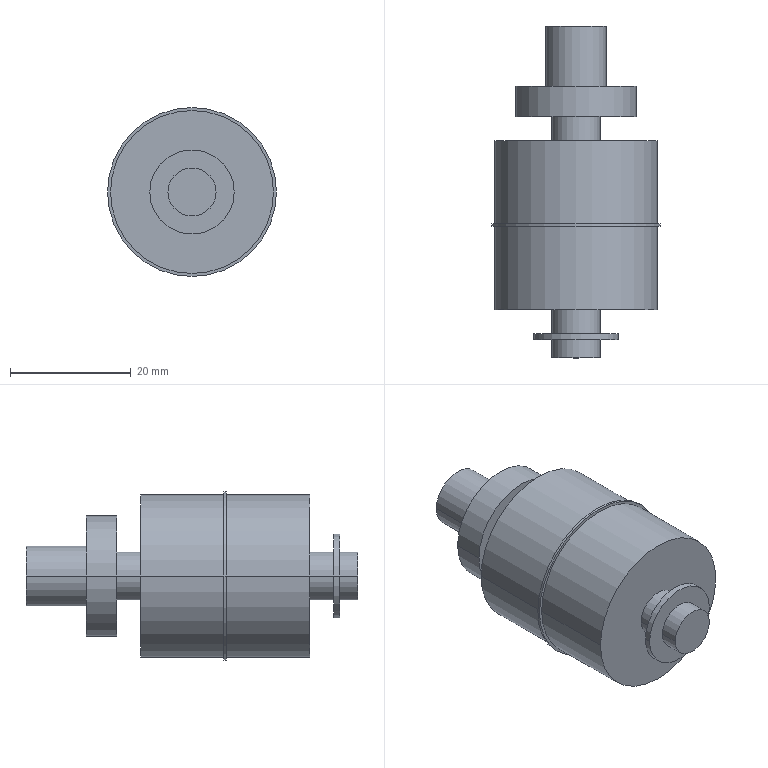Part | SolidWorks | features Revolution 1 | 1 solid | 28 faces | box 28 x 55 x 28 mm | volume 19112 mm3 | cylinder 18 | plane 10 | commonest cylinder face diameters 8 x6 27 x4 10 x2 14 x2 20 x2 28 x2
STEP:
#1=CARTESIAN_POINT('',(14.,22.2,0.));
#2=VERTEX_POINT('',#1);
#3=CARTESIAN_POINT('',(-14.,22.2,0.));
#4=VERTEX_POINT('',#3);
#5=CARTESIAN_POINT('',(0.,22.2,0.));
#6=DIRECTION('',(0.,-1.,0.));
#7=DIRECTION('',(1.,0.,0.));
#8=AXIS2_PLACEMENT_3D('',#5,#6,#7);
#9=CIRCLE('',#8,14.);
#10=EDGE_CURVE('',#2,#4,#9,.T.);
#11=ORIENTED_EDGE('',*,*,#10,.T.);
#12=CARTESIAN_POINT('',(-14.,21.8,0.));
#13=VERTEX_POINT('',#12);
#14=CARTESIAN_POINT('',(-14.,0.,0.));
#15=DIRECTION('',(0.,-1.,0.));
#16=VECTOR('',#15,1000.);
#17=LINE('',#14,#16);
#18=EDGE_CURVE('',#4,#13,#17,.T.);
#19=ORIENTED_EDGE('',*,*,#18,.T.);
#20=CARTESIAN_POINT('',(14.,21.8,0.));
#21=VERTEX_POINT('',#20);
#22=CARTESIAN_POINT('',(0.,21.8,0.));
#23=DIRECTION('',(0.,-1.,0.));
#24=DIRECTION('',(1.,0.,0.));
#25=AXIS2_PLACEMENT_3D('',#22,#23,#24);
#26=CIRCLE('',#25,14.);
#27=EDGE_CURVE('',#21,#13,#26,.T.);
#28=ORIENTED_EDGE('',*,*,#27,.F.);
#29=CARTESIAN_POINT('',(14.,0.,0.));
#30=DIRECTION('',(0.,-1.,0.));
#31=VECTOR('',#30,1000.);
#32=LINE('',#29,#31);
#33=EDGE_CURVE('',#2,#21,#32,.T.);
#34=ORIENTED_EDGE('',*,*,#33,.F.);
#35=EDGE_LOOP('',(#11,#19,#28,#34));
#36=FACE_OUTER_BOUND('',#35,.T.);
#37=CARTESIAN_POINT('',(0.,0.,0.));
#38=DIRECTION('',(0.,-1.,0.));
#39=DIRECTION('',(1.,0.,0.));
#40=AXIS2_PLACEMENT_3D('',#37,#38,#39);
#41=CYLINDRICAL_SURFACE('',#40,14.);
#42=ADVANCED_FACE('',(#36),#41,.T.);
#43=CARTESIAN_POINT('',(13.5,36.,0.));
#44=VERTEX_POINT('',#43);
#45=CARTESIAN_POINT('',(-13.5,36.,0.));
#46=VERTEX_POINT('',#45);
#47=CARTESIAN_POINT('',(0.,36.,0.));
#48=DIRECTION('',(0.,-1.,0.));
#49=DIRECTION('',(1.,0.,0.));
#50=AXIS2_PLACEMENT_3D('',#47,#48,#49);
#51=CIRCLE('',#50,13.5);
#52=EDGE_CURVE('',#44,#46,#51,.T.);
#53=ORIENTED_EDGE('',*,*,#52,.T.);
#54=CARTESIAN_POINT('',(-13.5,22.2,0.));
#55=VERTEX_POINT('',#54);
#56=CARTESIAN_POINT('',(-13.5,0.,0.));
#57=DIRECTION('',(0.,-1.,0.));
#58=VECTOR('',#57,1000.);
#59=LINE('',#56,#58);
#60=EDGE_CURVE('',#46,#55,#59,.T.);
#61=ORIENTED_EDGE('',*,*,#60,.T.);
#62=CARTESIAN_POINT('',(13.5,22.2,0.));
#63=VERTEX_POINT('',#62);
#64=CARTESIAN_POINT('',(0.,22.2,0.));
#65=DIRECTION('',(0.,-1.,0.));
#66=DIRECTION('',(1.,0.,0.));
#67=AXIS2_PLACEMENT_3D('',#64,#65,#66);
#68=CIRCLE('',#67,13.5);
#69=EDGE_CURVE('',#63,#55,#68,.T.);
#70=ORIENTED_EDGE('',*,*,#69,.F.);
#71=CARTESIAN_POINT('',(13.5,0.,0.));
#72=DIRECTION('',(0.,-1.,0.));
#73=VECTOR('',#72,1000.);
#74=LINE('',#71,#73);
#75=EDGE_CURVE('',#44,#63,#74,.T.);
#76=ORIENTED_EDGE('',*,*,#75,.F.);
#77=EDGE_LOOP('',(#53,#61,#70,#76));
#78=FACE_OUTER_BOUND('',#77,.T.);
#79=CARTESIAN_POINT('',(0.,0.,0.));
#80=DIRECTION('',(0.,-1.,0.));
#81=DIRECTION('',(1.,0.,0.));
#82=AXIS2_PLACEMENT_3D('',#79,#80,#81);
#83=CYLINDRICAL_SURFACE('',#82,13.5);
#84=ADVANCED_FACE('',(#78),#83,.T.);
#85=CARTESIAN_POINT('',(4.,40.,0.));
#86=VERTEX_POINT('',#85);
#87=CARTESIAN_POINT('',(-4.,40.,0.));
#88=VERTEX_POINT('',#87);
#89=CARTESIAN_POINT('',(0.,40.,0.));
#90=DIRECTION('',(0.,-1.,0.));
#91=DIRECTION('',(1.,0.,0.));
#92=AXIS2_PLACEMENT_3D('',#89,#90,#91);
#93=CIRCLE('',#92,4.);
#94=EDGE_CURVE('',#86,#88,#93,.T.);
#95=ORIENTED_EDGE('',*,*,#94,.T.);
#96=CARTESIAN_POINT('',(-4.,36.,0.));
#97=VERTEX_POINT('',#96);
#98=CARTESIAN_POINT('',(-4.,0.,0.));
#99=DIRECTION('',(0.,-1.,0.));
#100=VECTOR('',#99,1000.);
#101=LINE('',#98,#100);
#102=EDGE_CURVE('',#88,#97,#101,.T.);
#103=ORIENTED_EDGE('',*,*,#102,.T.);
#104=CARTESIAN_POINT('',(4.,36.,0.));
#105=VERTEX_POINT('',#104);
#106=CARTESIAN_POINT('',(0.,36.,0.));
#107=DIRECTION('',(0.,-1.,0.));
#108=DIRECTION('',(1.,0.,0.));
#109=AXIS2_PLACEMENT_3D('',#106,#107,#108);
#110=CIRCLE('',#109,4.);
#111=EDGE_CURVE('',#105,#97,#110,.T.);
#112=ORIENTED_EDGE('',*,*,#111,.F.);
#113=CARTESIAN_POINT('',(4.,0.,0.));
#114=DIRECTION('',(0.,-1.,0.));
#115=VECTOR('',#114,1000.);
#116=LINE('',#113,#115);
#117=EDGE_CURVE('',#86,#105,#116,.T.);
#118=ORIENTED_EDGE('',*,*,#117,.F.);
#119=EDGE_LOOP('',(#95,#103,#112,#118));
#120=FACE_OUTER_BOUND('',#119,.T.);
#121=CARTESIAN_POINT('',(0.,0.,0.));
#122=DIRECTION('',(0.,-1.,0.));
#123=DIRECTION('',(1.,0.,0.));
#124=AXIS2_PLACEMENT_3D('',#121,#122,#123);
#125=CYLINDRICAL_SURFACE('',#124,4.);
#126=ADVANCED_FACE('',(#120),#125,.T.);
#127=CARTESIAN_POINT('',(10.,45.,0.));
#128=VERTEX_POINT('',#127);
#129=CARTESIAN_POINT('',(-10.,45.,0.));
#130=VERTEX_POINT('',#129);
#131=CARTESIAN_POINT('',(0.,45.,0.));
#132=DIRECTION('',(0.,-1.,0.));
#133=DIRECTION('',(1.,0.,0.));
#134=AXIS2_PLACEMENT_3D('',#131,#132,#133);
#135=CIRCLE('',#134,10.);
#136=EDGE_CURVE('',#128,#130,#135,.T.);
#137=ORIENTED_EDGE('',*,*,#136,.T.);
#138=CARTESIAN_POINT('',(-10.,40.,0.));
#139=VERTEX_POINT('',#138);
#140=CARTESIAN_POINT('',(-10.,0.,0.));
#141=DIRECTION('',(0.,-1.,0.));
#142=VECTOR('',#141,1000.);
#143=LINE('',#140,#142);
#144=EDGE_CURVE('',#130,#139,#143,.T.);
#145=ORIENTED_EDGE('',*,*,#144,.T.);
#146=CARTESIAN_POINT('',(10.,40.,0.));
#147=VERTEX_POINT('',#146);
#148=CARTESIAN_POINT('',(0.,40.,0.));
#149=DIRECTION('',(0.,-1.,0.));
#150=DIRECTION('',(1.,0.,0.));
#151=AXIS2_PLACEMENT_3D('',#148,#149,#150);
#152=CIRCLE('',#151,10.);
#153=EDGE_CURVE('',#147,#139,#152,.T.);
#154=ORIENTED_EDGE('',*,*,#153,.F.);
#155=CARTESIAN_POINT('',(10.,0.,0.));
#156=DIRECTION('',(0.,-1.,0.));
#157=VECTOR('',#156,1000.);
#158=LINE('',#155,#157);
#159=EDGE_CURVE('',#128,#147,#158,.T.);
#160=ORIENTED_EDGE('',*,*,#159,.F.);
#161=EDGE_LOOP('',(#137,#145,#154,#160));
#162=FACE_OUTER_BOUND('',#161,.T.);
#163=CARTESIAN_POINT('',(0.,0.,0.));
#164=DIRECTION('',(0.,-1.,0.));
#165=DIRECTION('',(1.,0.,0.));
#166=AXIS2_PLACEMENT_3D('',#163,#164,#165);
#167=CYLINDRICAL_SURFACE('',#166,10.);
#168=ADVANCED_FACE('',(#162),#167,.T.);
#169=CARTESIAN_POINT('',(5.,55.,0.));
#170=VERTEX_POINT('',#169);
#171=CARTESIAN_POINT('',(-5.,55.,0.));
#172=VERTEX_POINT('',#171);
#173=CARTESIAN_POINT('',(0.,55.,0.));
#174=DIRECTION('',(0.,-1.,0.));
#175=DIRECTION('',(1.,0.,0.));
#176=AXIS2_PLACEMENT_3D('',#173,#174,#175);
#177=CIRCLE('',#176,5.);
#178=EDGE_CURVE('',#170,#172,#177,.T.);
#179=ORIENTED_EDGE('',*,*,#178,.T.);
#180=CARTESIAN_POINT('',(-5.,45.,0.));
#181=VERTEX_POINT('',#180);
#182=CARTESIAN_POINT('',(-5.,0.,0.));
#183=DIRECTION('',(0.,-1.,0.));
#184=VECTOR('',#183,1000.);
#185=LINE('',#182,#184);
#186=EDGE_CURVE('',#172,#181,#185,.T.);
#187=ORIENTED_EDGE('',*,*,#186,.T.);
#188=CARTESIAN_POINT('',(5.,45.,0.));
#189=VERTEX_POINT('',#188);
#190=CARTESIAN_POINT('',(0.,45.,0.));
#191=DIRECTION('',(0.,-1.,0.));
#192=DIRECTION('',(1.,0.,0.));
#193=AXIS2_PLACEMENT_3D('',#190,#191,#192);
#194=CIRCLE('',#193,5.);
#195=EDGE_CURVE('',#189,#181,#194,.T.);
#196=ORIENTED_EDGE('',*,*,#195,.F.);
#197=CARTESIAN_POINT('',(5.,0.,0.));
#198=DIRECTION('',(0.,-1.,0.));
#199=VECTOR('',#198,1000.);
#200=LINE('',#197,#199);
#201=EDGE_CURVE('',#170,#189,#200,.T.);
#202=ORIENTED_EDGE('',*,*,#201,.F.);
#203=EDGE_LOOP('',(#179,#187,#196,#202));
#204=FACE_OUTER_BOUND('',#203,.T.);
#205=CARTESIAN_POINT('',(0.,0.,0.));
#206=DIRECTION('',(0.,-1.,0.));
#207=DIRECTION('',(1.,0.,0.));
#208=AXIS2_PLACEMENT_3D('',#205,#206,#207);
#209=CYLINDRICAL_SURFACE('',#208,5.);
#210=ADVANCED_FACE('',(#204),#209,.T.);
#211=CARTESIAN_POINT('',(4.,3.,0.));
#212=VERTEX_POINT('',#211);
#213=CARTESIAN_POINT('',(-4.,3.,0.));
#214=VERTEX_POINT('',#213);
#215=CARTESIAN_POINT('',(0.,3.,0.));
#216=DIRECTION('',(0.,-1.,0.));
#217=DIRECTION('',(1.,0.,0.));
#218=AXIS2_PLACEMENT_3D('',#215,#216,#217);
#219=CIRCLE('',#218,4.);
#220=EDGE_CURVE('',#212,#214,#219,.T.);
#221=ORIENTED_EDGE('',*,*,#220,.T.);
#222=CARTESIAN_POINT('',(-4.,0.,0.));
#223=VERTEX_POINT('',#222);
#224=CARTESIAN_POINT('',(-4.,0.,0.));
#225=DIRECTION('',(0.,-1.,0.));
#226=VECTOR('',#225,1000.);
#227=LINE('',#224,#226);
#228=EDGE_CURVE('',#214,#223,#227,.T.);
#229=ORIENTED_EDGE('',*,*,#228,.T.);
#230=CARTESIAN_POINT('',(4.,0.,0.));
#231=VERTEX_POINT('',#230);
#232=CARTESIAN_POINT('',(0.,0.,0.));
#233=DIRECTION('',(0.,-1.,0.));
#234=DIRECTION('',(1.,0.,0.));
#235=AXIS2_PLACEMENT_3D('',#232,#233,#234);
#236=CIRCLE('',#235,4.);
#237=EDGE_CURVE('',#231,#223,#236,.T.);
#238=ORIENTED_EDGE('',*,*,#237,.F.);
#239=CARTESIAN_POINT('',(4.,0.,0.));
#240=DIRECTION('',(0.,-1.,0.));
#241=VECTOR('',#240,1000.);
#242=LINE('',#239,#241);
#243=EDGE_CURVE('',#212,#231,#242,.T.);
#244=ORIENTED_EDGE('',*,*,#243,.F.);
#245=EDGE_LOOP('',(#221,#229,#238,#244));
#246=FACE_OUTER_BOUND('',#245,.T.);
#247=CARTESIAN_POINT('',(0.,0.,0.));
#248=DIRECTION('',(0.,-1.,0.));
#249=DIRECTION('',(1.,0.,0.));
#250=AXIS2_PLACEMENT_3D('',#247,#248,#249);
#251=CYLINDRICAL_SURFACE('',#250,4.);
#252=ADVANCED_FACE('',(#246),#251,.T.);
#253=CARTESIAN_POINT('',(7.,4.,0.));
#254=VERTEX_POINT('',#253);
#255=CARTESIAN_POINT('',(-7.,4.,0.));
#256=VERTEX_POINT('',#255);
#257=CARTESIAN_POINT('',(0.,4.,0.));
#258=DIRECTION('',(0.,-1.,0.));
#259=DIRECTION('',(1.,0.,0.));
#260=AXIS2_PLACEMENT_3D('',#257,#258,#259);
#261=CIRCLE('',#260,7.);
#262=EDGE_CURVE('',#254,#256,#261,.T.);
#263=ORIENTED_EDGE('',*,*,#262,.T.);
#264=CARTESIAN_POINT('',(-7.,3.,0.));
#265=VERTEX_POINT('',#264);
#266=CARTESIAN_POINT('',(-7.,0.,0.));
#267=DIRECTION('',(0.,-1.,0.));
#268=VECTOR('',#267,1000.);
#269=LINE('',#266,#268);
#270=EDGE_CURVE('',#256,#265,#269,.T.);
#271=ORIENTED_EDGE('',*,*,#270,.T.);
#272=CARTESIAN_POINT('',(7.,3.,0.));
#273=VERTEX_POINT('',#272);
#274=CARTESIAN_POINT('',(0.,3.,0.));
#275=DIRECTION('',(0.,-1.,0.));
#276=DIRECTION('',(1.,0.,0.));
#277=AXIS2_PLACEMENT_3D('',#274,#275,#276);
#278=CIRCLE('',#277,7.);
#279=EDGE_CURVE('',#273,#265,#278,.T.);
#280=ORIENTED_EDGE('',*,*,#279,.F.);
#281=CARTESIAN_POINT('',(7.,0.,0.));
#282=DIRECTION('',(0.,-1.,0.));
#283=VECTOR('',#282,1000.);
#284=LINE('',#281,#283);
#285=EDGE_CURVE('',#254,#273,#284,.T.);
#286=ORIENTED_EDGE('',*,*,#285,.F.);
#287=EDGE_LOOP('',(#263,#271,#280,#286));
#288=FACE_OUTER_BOUND('',#287,.T.);
#289=CARTESIAN_POINT('',(0.,0.,0.));
#290=DIRECTION('',(0.,-1.,0.));
#291=DIRECTION('',(1.,0.,0.));
#292=AXIS2_PLACEMENT_3D('',#289,#290,#291);
#293=CYLINDRICAL_SURFACE('',#292,7.);
#294=ADVANCED_FACE('',(#288),#293,.T.);
#295=CARTESIAN_POINT('',(4.,8.,0.));
#296=VERTEX_POINT('',#295);
#297=CARTESIAN_POINT('',(-4.,8.,0.));
#298=VERTEX_POINT('',#297);
#299=CARTESIAN_POINT('',(0.,8.,0.));
#300=DIRECTION('',(0.,-1.,0.));
#301=DIRECTION('',(1.,0.,0.));
#302=AXIS2_PLACEMENT_3D('',#299,#300,#301);
#303=CIRCLE('',#302,4.);
#304=EDGE_CURVE('',#296,#298,#303,.T.);
#305=ORIENTED_EDGE('',*,*,#304,.T.);
#306=CARTESIAN_POINT('',(-4.,4.,0.));
#307=VERTEX_POINT('',#306);
#308=CARTESIAN_POINT('',(-4.,0.,0.));
#309=DIRECTION('',(0.,-1.,0.));
#310=VECTOR('',#309,1000.);
#311=LINE('',#308,#310);
#312=EDGE_CURVE('',#298,#307,#311,.T.);
#313=ORIENTED_EDGE('',*,*,#312,.T.);
#314=CARTESIAN_POINT('',(4.,4.,0.));
#315=VERTEX_POINT('',#314);
#316=CARTESIAN_POINT('',(0.,4.,0.));
#317=DIRECTION('',(0.,-1.,0.));
#318=DIRECTION('',(1.,0.,0.));
#319=AXIS2_PLACEMENT_3D('',#316,#317,#318);
#320=CIRCLE('',#319,4.);
#321=EDGE_CURVE('',#315,#307,#320,.T.);
#322=ORIENTED_EDGE('',*,*,#321,.F.);
#323=CARTESIAN_POINT('',(4.,0.,0.));
#324=DIRECTION('',(0.,-1.,0.));
#325=VECTOR('',#324,1000.);
#326=LINE('',#323,#325);
#327=EDGE_CURVE('',#296,#315,#326,.T.);
#328=ORIENTED_EDGE('',*,*,#327,.F.);
#329=EDGE_LOOP('',(#305,#313,#322,#328));
#330=FACE_OUTER_BOUND('',#329,.T.);
#331=CARTESIAN_POINT('',(0.,0.,0.));
#332=DIRECTION('',(0.,-1.,0.));
#333=DIRECTION('',(1.,0.,0.));
#334=AXIS2_PLACEMENT_3D('',#331,#332,#333);
#335=CYLINDRICAL_SURFACE('',#334,4.);
#336=ADVANCED_FACE('',(#330),#335,.T.);
#337=CARTESIAN_POINT('',(13.5,21.8,0.));
#338=VERTEX_POINT('',#337);
#339=CARTESIAN_POINT('',(-13.5,21.8,0.));
#340=VERTEX_POINT('',#339);
#341=CARTESIAN_POINT('',(0.,21.8,0.));
#342=DIRECTION('',(0.,-1.,0.));
#343=DIRECTION('',(1.,0.,0.));
#344=AXIS2_PLACEMENT_3D('',#341,#342,#343);
#345=CIRCLE('',#344,13.5);
#346=EDGE_CURVE('',#338,#340,#345,.T.);
#347=ORIENTED_EDGE('',*,*,#346,.T.);
#348=CARTESIAN_POINT('',(-13.5,8.,0.));
#349=VERTEX_POINT('',#348);
#350=CARTESIAN_POINT('',(-13.5,0.,0.));
#351=DIRECTION('',(0.,-1.,0.));
#352=VECTOR('',#351,1000.);
#353=LINE('',#350,#352);
#354=EDGE_CURVE('',#340,#349,#353,.T.);
#355=ORIENTED_EDGE('',*,*,#354,.T.);
#356=CARTESIAN_POINT('',(13.5,8.,0.));
#357=VERTEX_POINT('',#356);
#358=CARTESIAN_POINT('',(0.,8.,0.));
#359=DIRECTION('',(0.,-1.,0.));
#360=DIRECTION('',(1.,0.,0.));
#361=AXIS2_PLACEMENT_3D('',#358,#359,#360);
#362=CIRCLE('',#361,13.5);
#363=EDGE_CURVE('',#357,#349,#362,.T.);
#364=ORIENTED_EDGE('',*,*,#363,.F.);
#365=CARTESIAN_POINT('',(13.5,0.,0.));
#366=DIRECTION('',(0.,-1.,0.));
#367=VECTOR('',#366,1000.);
#368=LINE('',#365,#367);
#369=EDGE_CURVE('',#338,#357,#368,.T.);
#370=ORIENTED_EDGE('',*,*,#369,.F.);
#371=EDGE_LOOP('',(#347,#355,#364,#370));
#372=FACE_OUTER_BOUND('',#371,.T.);
#373=CARTESIAN_POINT('',(0.,0.,0.));
#374=DIRECTION('',(0.,-1.,0.));
#375=DIRECTION('',(1.,0.,0.));
#376=AXIS2_PLACEMENT_3D('',#373,#374,#375);
#377=CYLINDRICAL_SURFACE('',#376,13.5);
#378=ADVANCED_FACE('',(#372),#377,.T.);
#379=ORIENTED_EDGE('',*,*,#346,.F.);
#380=CARTESIAN_POINT('',(0.,21.8,0.));
#381=DIRECTION('',(0.,-1.,0.));
#382=DIRECTION('',(1.,0.,0.));
#383=AXIS2_PLACEMENT_3D('',#380,#381,#382);
#384=CIRCLE('',#383,13.5);
#385=EDGE_CURVE('',#340,#338,#384,.T.);
#386=ORIENTED_EDGE('',*,*,#385,.F.);
#387=EDGE_LOOP('',(#379,#386));
#388=FACE_BOUND('',#387,.T.);
#389=ORIENTED_EDGE('',*,*,#27,.T.);
#390=CARTESIAN_POINT('',(0.,21.8,0.));
#391=DIRECTION('',(0.,-1.,0.));
#392=DIRECTION('',(1.,0.,0.));
#393=AXIS2_PLACEMENT_3D('',#390,#391,#392);
#394=CIRCLE('',#393,14.);
#395=EDGE_CURVE('',#13,#21,#394,.T.);
#396=ORIENTED_EDGE('',*,*,#395,.T.);
#397=EDGE_LOOP('',(#389,#396));
#398=FACE_OUTER_BOUND('',#397,.T.);
#399=CARTESIAN_POINT('',(0.,21.8,0.));
#400=DIRECTION('',(0.,1.,0.));
#401=DIRECTION('',(-1.,0.,0.));
#402=AXIS2_PLACEMENT_3D('',#399,#400,#401);
#403=PLANE('',#402);
#404=ADVANCED_FACE('',(#388,#398),#403,.F.);
#405=ORIENTED_EDGE('',*,*,#354,.F.);
#406=ORIENTED_EDGE('',*,*,#385,.T.);
#407=ORIENTED_EDGE('',*,*,#369,.T.);
#408=CARTESIAN_POINT('',(0.,8.,0.));
#409=DIRECTION('',(0.,-1.,0.));
#410=DIRECTION('',(1.,0.,0.));
#411=AXIS2_PLACEMENT_3D('',#408,#409,#410);
#412=CIRCLE('',#411,13.5);
#413=EDGE_CURVE('',#349,#357,#412,.T.);
#414=ORIENTED_EDGE('',*,*,#413,.F.);
#415=EDGE_LOOP('',(#405,#406,#407,#414));
#416=FACE_OUTER_BOUND('',#415,.T.);
#417=CARTESIAN_POINT('',(0.,0.,0.));
#418=DIRECTION('',(0.,-1.,0.));
#419=DIRECTION('',(1.,0.,0.));
#420=AXIS2_PLACEMENT_3D('',#417,#418,#419);
#421=CYLINDRICAL_SURFACE('',#420,13.5);
#422=ADVANCED_FACE('',(#416),#421,.T.);
#423=ORIENTED_EDGE('',*,*,#304,.F.);
#424=CARTESIAN_POINT('',(0.,8.,0.));
#425=DIRECTION('',(0.,-1.,0.));
#426=DIRECTION('',(1.,0.,0.));
#427=AXIS2_PLACEMENT_3D('',#424,#425,#426);
#428=CIRCLE('',#427,4.);
#429=EDGE_CURVE('',#298,#296,#428,.T.);
#430=ORIENTED_EDGE('',*,*,#429,.F.);
#431=EDGE_LOOP('',(#423,#430));
#432=FACE_BOUND('',#431,.T.);
#433=ORIENTED_EDGE('',*,*,#363,.T.);
#434=ORIENTED_EDGE('',*,*,#413,.T.);
#435=EDGE_LOOP('',(#433,#434));
#436=FACE_OUTER_BOUND('',#435,.T.);
#437=CARTESIAN_POINT('',(0.,8.,0.));
#438=DIRECTION('',(0.,1.,0.));
#439=DIRECTION('',(-1.,0.,0.));
#440=AXIS2_PLACEMENT_3D('',#437,#438,#439);
#441=PLANE('',#440);
#442=ADVANCED_FACE('',(#432,#436),#441,.F.);
#443=ORIENTED_EDGE('',*,*,#312,.F.);
#444=ORIENTED_EDGE('',*,*,#429,.T.);
#445=ORIENTED_EDGE('',*,*,#327,.T.);
#446=CARTESIAN_POINT('',(0.,4.,0.));
#447=DIRECTION('',(0.,-1.,0.));
#448=DIRECTION('',(1.,0.,0.));
#449=AXIS2_PLACEMENT_3D('',#446,#447,#448);
#450=CIRCLE('',#449,4.);
#451=EDGE_CURVE('',#307,#315,#450,.T.);
#452=ORIENTED_EDGE('',*,*,#451,.F.);
#453=EDGE_LOOP('',(#443,#444,#445,#452));
#454=FACE_OUTER_BOUND('',#453,.T.);
#455=CARTESIAN_POINT('',(0.,0.,0.));
#456=DIRECTION('',(0.,-1.,0.));
#457=DIRECTION('',(1.,0.,0.));
#458=AXIS2_PLACEMENT_3D('',#455,#456,#457);
#459=CYLINDRICAL_SURFACE('',#458,4.);
#460=ADVANCED_FACE('',(#454),#459,.T.);
#461=ORIENTED_EDGE('',*,*,#262,.F.);
#462=CARTESIAN_POINT('',(0.,4.,0.));
#463=DIRECTION('',(0.,-1.,0.));
#464=DIRECTION('',(1.,0.,0.));
#465=AXIS2_PLACEMENT_3D('',#462,#463,#464);
#466=CIRCLE('',#465,7.);
#467=EDGE_CURVE('',#256,#254,#466,.T.);
#468=ORIENTED_EDGE('',*,*,#467,.F.);
#469=EDGE_LOOP('',(#461,#468));
#470=FACE_OUTER_BOUND('',#469,.T.);
#471=ORIENTED_EDGE('',*,*,#321,.T.);
#472=ORIENTED_EDGE('',*,*,#451,.T.);
#473=EDGE_LOOP('',(#471,#472));
#474=FACE_BOUND('',#473,.T.);
#475=CARTESIAN_POINT('',(0.,4.,0.));
#476=DIRECTION('',(0.,-1.,0.));
#477=DIRECTION('',(1.,0.,0.));
#478=AXIS2_PLACEMENT_3D('',#475,#476,#477);
#479=PLANE('',#478);
#480=ADVANCED_FACE('',(#470,#474),#479,.F.);
#481=ORIENTED_EDGE('',*,*,#270,.F.);
#482=ORIENTED_EDGE('',*,*,#467,.T.);
#483=ORIENTED_EDGE('',*,*,#285,.T.);
#484=CARTESIAN_POINT('',(0.,3.,0.));
#485=DIRECTION('',(0.,-1.,0.));
#486=DIRECTION('',(1.,0.,0.));
#487=AXIS2_PLACEMENT_3D('',#484,#485,#486);
#488=CIRCLE('',#487,7.);
#489=EDGE_CURVE('',#265,#273,#488,.T.);
#490=ORIENTED_EDGE('',*,*,#489,.F.);
#491=EDGE_LOOP('',(#481,#482,#483,#490));
#492=FACE_OUTER_BOUND('',#491,.T.);
#493=CARTESIAN_POINT('',(0.,0.,0.));
#494=DIRECTION('',(0.,-1.,0.));
#495=DIRECTION('',(1.,0.,0.));
#496=AXIS2_PLACEMENT_3D('',#493,#494,#495);
#497=CYLINDRICAL_SURFACE('',#496,7.);
#498=ADVANCED_FACE('',(#492),#497,.T.);
#499=ORIENTED_EDGE('',*,*,#220,.F.);
#500=CARTESIAN_POINT('',(0.,3.,0.));
#501=DIRECTION('',(0.,-1.,0.));
#502=DIRECTION('',(1.,0.,0.));
#503=AXIS2_PLACEMENT_3D('',#500,#501,#502);
#504=CIRCLE('',#503,4.);
#505=EDGE_CURVE('',#214,#212,#504,.T.);
#506=ORIENTED_EDGE('',*,*,#505,.F.);
#507=EDGE_LOOP('',(#499,#506));
#508=FACE_BOUND('',#507,.T.);
#509=ORIENTED_EDGE('',*,*,#279,.T.);
#510=ORIENTED_EDGE('',*,*,#489,.T.);
#511=EDGE_LOOP('',(#509,#510));
#512=FACE_OUTER_BOUND('',#511,.T.);
#513=CARTESIAN_POINT('',(0.,3.,0.));
#514=DIRECTION('',(0.,1.,0.));
#515=DIRECTION('',(-1.,0.,0.));
#516=AXIS2_PLACEMENT_3D('',#513,#514,#515);
#517=PLANE('',#516);
#518=ADVANCED_FACE('',(#508,#512),#517,.F.);
#519=ORIENTED_EDGE('',*,*,#228,.F.);
#520=ORIENTED_EDGE('',*,*,#505,.T.);
#521=ORIENTED_EDGE('',*,*,#243,.T.);
#522=CARTESIAN_POINT('',(0.,0.,0.));
#523=DIRECTION('',(0.,-1.,0.));
#524=DIRECTION('',(1.,0.,0.));
#525=AXIS2_PLACEMENT_3D('',#522,#523,#524);
#526=CIRCLE('',#525,4.);
#527=EDGE_CURVE('',#223,#231,#526,.T.);
#528=ORIENTED_EDGE('',*,*,#527,.F.);
#529=EDGE_LOOP('',(#519,#520,#521,#528));
#530=FACE_OUTER_BOUND('',#529,.T.);
#531=CARTESIAN_POINT('',(0.,0.,0.));
#532=DIRECTION('',(0.,-1.,0.));
#533=DIRECTION('',(1.,0.,0.));
#534=AXIS2_PLACEMENT_3D('',#531,#532,#533);
#535=CYLINDRICAL_SURFACE('',#534,4.);
#536=ADVANCED_FACE('',(#530),#535,.T.);
#537=ORIENTED_EDGE('',*,*,#237,.T.);
#538=ORIENTED_EDGE('',*,*,#527,.T.);
#539=EDGE_LOOP('',(#537,#538));
#540=FACE_OUTER_BOUND('',#539,.T.);
#541=CARTESIAN_POINT('',(0.,0.,0.));
#542=DIRECTION('',(0.,1.,0.));
#543=DIRECTION('',(-1.,0.,0.));
#544=AXIS2_PLACEMENT_3D('',#541,#542,#543);
#545=PLANE('',#544);
#546=ADVANCED_FACE('',(#540),#545,.F.);
#547=ORIENTED_EDGE('',*,*,#178,.F.);
#548=CARTESIAN_POINT('',(0.,55.,0.));
#549=DIRECTION('',(0.,-1.,0.));
#550=DIRECTION('',(1.,0.,0.));
#551=AXIS2_PLACEMENT_3D('',#548,#549,#550);
#552=CIRCLE('',#551,5.);
#553=EDGE_CURVE('',#172,#170,#552,.T.);
#554=ORIENTED_EDGE('',*,*,#553,.F.);
#555=EDGE_LOOP('',(#547,#554));
#556=FACE_OUTER_BOUND('',#555,.T.);
#557=CARTESIAN_POINT('',(0.,55.,0.));
#558=DIRECTION('',(0.,-1.,0.));
#559=DIRECTION('',(1.,0.,0.));
#560=AXIS2_PLACEMENT_3D('',#557,#558,#559);
#561=PLANE('',#560);
#562=ADVANCED_FACE('',(#556),#561,.F.);
#563=ORIENTED_EDGE('',*,*,#186,.F.);
#564=ORIENTED_EDGE('',*,*,#553,.T.);
#565=ORIENTED_EDGE('',*,*,#201,.T.);
#566=CARTESIAN_POINT('',(0.,45.,0.));
#567=DIRECTION('',(0.,-1.,0.));
#568=DIRECTION('',(1.,0.,0.));
#569=AXIS2_PLACEMENT_3D('',#566,#567,#568);
#570=CIRCLE('',#569,5.);
#571=EDGE_CURVE('',#181,#189,#570,.T.);
#572=ORIENTED_EDGE('',*,*,#571,.F.);
#573=EDGE_LOOP('',(#563,#564,#565,#572));
#574=FACE_OUTER_BOUND('',#573,.T.);
#575=CARTESIAN_POINT('',(0.,0.,0.));
#576=DIRECTION('',(0.,-1.,0.));
#577=DIRECTION('',(1.,0.,0.));
#578=AXIS2_PLACEMENT_3D('',#575,#576,#577);
#579=CYLINDRICAL_SURFACE('',#578,5.);
#580=ADVANCED_FACE('',(#574),#579,.T.);
#581=ORIENTED_EDGE('',*,*,#136,.F.);
#582=CARTESIAN_POINT('',(0.,45.,0.));
#583=DIRECTION('',(0.,-1.,0.));
#584=DIRECTION('',(1.,0.,0.));
#585=AXIS2_PLACEMENT_3D('',#582,#583,#584);
#586=CIRCLE('',#585,10.);
#587=EDGE_CURVE('',#130,#128,#586,.T.);
#588=ORIENTED_EDGE('',*,*,#587,.F.);
#589=EDGE_LOOP('',(#581,#588));
#590=FACE_OUTER_BOUND('',#589,.T.);
#591=ORIENTED_EDGE('',*,*,#195,.T.);
#592=ORIENTED_EDGE('',*,*,#571,.T.);
#593=EDGE_LOOP('',(#591,#592));
#594=FACE_BOUND('',#593,.T.);
#595=CARTESIAN_POINT('',(0.,45.,0.));
#596=DIRECTION('',(0.,-1.,0.));
#597=DIRECTION('',(1.,0.,0.));
#598=AXIS2_PLACEMENT_3D('',#595,#596,#597);
#599=PLANE('',#598);
#600=ADVANCED_FACE('',(#590,#594),#599,.F.);
#601=ORIENTED_EDGE('',*,*,#144,.F.);
#602=ORIENTED_EDGE('',*,*,#587,.T.);
#603=ORIENTED_EDGE('',*,*,#159,.T.);
#604=CARTESIAN_POINT('',(0.,40.,0.));
#605=DIRECTION('',(0.,-1.,0.));
#606=DIRECTION('',(1.,0.,0.));
#607=AXIS2_PLACEMENT_3D('',#604,#605,#606);
#608=CIRCLE('',#607,10.);
#609=EDGE_CURVE('',#139,#147,#608,.T.);
#610=ORIENTED_EDGE('',*,*,#609,.F.);
#611=EDGE_LOOP('',(#601,#602,#603,#610));
#612=FACE_OUTER_BOUND('',#611,.T.);
#613=CARTESIAN_POINT('',(0.,0.,0.));
#614=DIRECTION('',(0.,-1.,0.));
#615=DIRECTION('',(1.,0.,0.));
#616=AXIS2_PLACEMENT_3D('',#613,#614,#615);
#617=CYLINDRICAL_SURFACE('',#616,10.);
#618=ADVANCED_FACE('',(#612),#617,.T.);
#619=ORIENTED_EDGE('',*,*,#94,.F.);
#620=CARTESIAN_POINT('',(0.,40.,0.));
#621=DIRECTION('',(0.,-1.,0.));
#622=DIRECTION('',(1.,0.,0.));
#623=AXIS2_PLACEMENT_3D('',#620,#621,#622);
#624=CIRCLE('',#623,4.);
#625=EDGE_CURVE('',#88,#86,#624,.T.);
#626=ORIENTED_EDGE('',*,*,#625,.F.);
#627=EDGE_LOOP('',(#619,#626));
#628=FACE_BOUND('',#627,.T.);
#629=ORIENTED_EDGE('',*,*,#153,.T.);
#630=ORIENTED_EDGE('',*,*,#609,.T.);
#631=EDGE_LOOP('',(#629,#630));
#632=FACE_OUTER_BOUND('',#631,.T.);
#633=CARTESIAN_POINT('',(0.,40.,0.));
#634=DIRECTION('',(0.,1.,0.));
#635=DIRECTION('',(-1.,0.,0.));
#636=AXIS2_PLACEMENT_3D('',#633,#634,#635);
#637=PLANE('',#636);
#638=ADVANCED_FACE('',(#628,#632),#637,.F.);
#639=ORIENTED_EDGE('',*,*,#102,.F.);
#640=ORIENTED_EDGE('',*,*,#625,.T.);
#641=ORIENTED_EDGE('',*,*,#117,.T.);
#642=CARTESIAN_POINT('',(0.,36.,0.));
#643=DIRECTION('',(0.,-1.,0.));
#644=DIRECTION('',(1.,0.,0.));
#645=AXIS2_PLACEMENT_3D('',#642,#643,#644);
#646=CIRCLE('',#645,4.);
#647=EDGE_CURVE('',#97,#105,#646,.T.);
#648=ORIENTED_EDGE('',*,*,#647,.F.);
#649=EDGE_LOOP('',(#639,#640,#641,#648));
#650=FACE_OUTER_BOUND('',#649,.T.);
#651=CARTESIAN_POINT('',(0.,0.,0.));
#652=DIRECTION('',(0.,-1.,0.));
#653=DIRECTION('',(1.,0.,0.));
#654=AXIS2_PLACEMENT_3D('',#651,#652,#653);
#655=CYLINDRICAL_SURFACE('',#654,4.);
#656=ADVANCED_FACE('',(#650),#655,.T.);
#657=ORIENTED_EDGE('',*,*,#52,.F.);
#658=CARTESIAN_POINT('',(0.,36.,0.));
#659=DIRECTION('',(0.,-1.,0.));
#660=DIRECTION('',(1.,0.,0.));
#661=AXIS2_PLACEMENT_3D('',#658,#659,#660);
#662=CIRCLE('',#661,13.5);
#663=EDGE_CURVE('',#46,#44,#662,.T.);
#664=ORIENTED_EDGE('',*,*,#663,.F.);
#665=EDGE_LOOP('',(#657,#664));
#666=FACE_OUTER_BOUND('',#665,.T.);
#667=ORIENTED_EDGE('',*,*,#111,.T.);
#668=ORIENTED_EDGE('',*,*,#647,.T.);
#669=EDGE_LOOP('',(#667,#668));
#670=FACE_BOUND('',#669,.T.);
#671=CARTESIAN_POINT('',(0.,36.,0.));
#672=DIRECTION('',(0.,-1.,0.));
#673=DIRECTION('',(1.,0.,0.));
#674=AXIS2_PLACEMENT_3D('',#671,#672,#673);
#675=PLANE('',#674);
#676=ADVANCED_FACE('',(#666,#670),#675,.F.);
#677=ORIENTED_EDGE('',*,*,#60,.F.);
#678=ORIENTED_EDGE('',*,*,#663,.T.);
#679=ORIENTED_EDGE('',*,*,#75,.T.);
#680=CARTESIAN_POINT('',(0.,22.2,0.));
#681=DIRECTION('',(0.,-1.,0.));
#682=DIRECTION('',(1.,0.,0.));
#683=AXIS2_PLACEMENT_3D('',#680,#681,#682);
#684=CIRCLE('',#683,13.5);
#685=EDGE_CURVE('',#55,#63,#684,.T.);
#686=ORIENTED_EDGE('',*,*,#685,.F.);
#687=EDGE_LOOP('',(#677,#678,#679,#686));
#688=FACE_OUTER_BOUND('',#687,.T.);
#689=CARTESIAN_POINT('',(0.,0.,0.));
#690=DIRECTION('',(0.,-1.,0.));
#691=DIRECTION('',(1.,0.,0.));
#692=AXIS2_PLACEMENT_3D('',#689,#690,#691);
#693=CYLINDRICAL_SURFACE('',#692,13.5);
#694=ADVANCED_FACE('',(#688),#693,.T.);
#695=ORIENTED_EDGE('',*,*,#10,.F.);
#696=CARTESIAN_POINT('',(0.,22.2,0.));
#697=DIRECTION('',(0.,-1.,0.));
#698=DIRECTION('',(1.,0.,0.));
#699=AXIS2_PLACEMENT_3D('',#696,#697,#698);
#700=CIRCLE('',#699,14.);
#701=EDGE_CURVE('',#4,#2,#700,.T.);
#702=ORIENTED_EDGE('',*,*,#701,.F.);
#703=EDGE_LOOP('',(#695,#702));
#704=FACE_OUTER_BOUND('',#703,.T.);
#705=ORIENTED_EDGE('',*,*,#69,.T.);
#706=ORIENTED_EDGE('',*,*,#685,.T.);
#707=EDGE_LOOP('',(#705,#706));
#708=FACE_BOUND('',#707,.T.);
#709=CARTESIAN_POINT('',(0.,22.2,0.));
#710=DIRECTION('',(0.,-1.,0.));
#711=DIRECTION('',(1.,0.,0.));
#712=AXIS2_PLACEMENT_3D('',#709,#710,#711);
#713=PLANE('',#712);
#714=ADVANCED_FACE('',(#704,#708),#713,.F.);
#715=ORIENTED_EDGE('',*,*,#18,.F.);
#716=ORIENTED_EDGE('',*,*,#701,.T.);
#717=ORIENTED_EDGE('',*,*,#33,.T.);
#718=ORIENTED_EDGE('',*,*,#395,.F.);
#719=EDGE_LOOP('',(#715,#716,#717,#718));
#720=FACE_OUTER_BOUND('',#719,.T.);
#721=CARTESIAN_POINT('',(0.,0.,0.));
#722=DIRECTION('',(0.,-1.,0.));
#723=DIRECTION('',(1.,0.,0.));
#724=AXIS2_PLACEMENT_3D('',#721,#722,#723);
#725=CYLINDRICAL_SURFACE('',#724,14.);
#726=ADVANCED_FACE('',(#720),#725,.T.);
#727=CLOSED_SHELL('',(#42,#84,#126,#168,#210,#252,#294,#336,#378,#404,#422,#442,#460,#480,#498,#518,#536,#546,#562,#580,#600,#618,#638,#656,#676,#694,#714,#726));
#728=MANIFOLD_SOLID_BREP('',#727);
#729=CARTESIAN_POINT('',(0.,0.,0.));
#730=DIRECTION('',(0.,0.,1.));
#731=DIRECTION('',(1.,0.,0.));
#732=AXIS2_PLACEMENT_3D('',#729,#730,#731);
#733=(LENGTH_UNIT()NAMED_UNIT(*)SI_UNIT(.MILLI.,.METRE.));
#734=UNCERTAINTY_MEASURE_WITH_UNIT(LENGTH_MEASURE(0.00001),#733,'','');
#735=(NAMED_UNIT(*)PLANE_ANGLE_UNIT()SI_UNIT($,.RADIAN.));
#736=(NAMED_UNIT(*)SI_UNIT($,.STERADIAN.)SOLID_ANGLE_UNIT());
#737=(GEOMETRIC_REPRESENTATION_CONTEXT(3)GLOBAL_UNCERTAINTY_ASSIGNED_CONTEXT((#734))GLOBAL_UNIT_ASSIGNED_CONTEXT((#733,#735,#736))REPRESENTATION_CONTEXT('',''));
#738=ADVANCED_BREP_SHAPE_REPRESENTATION('',(#728,#732),#737);